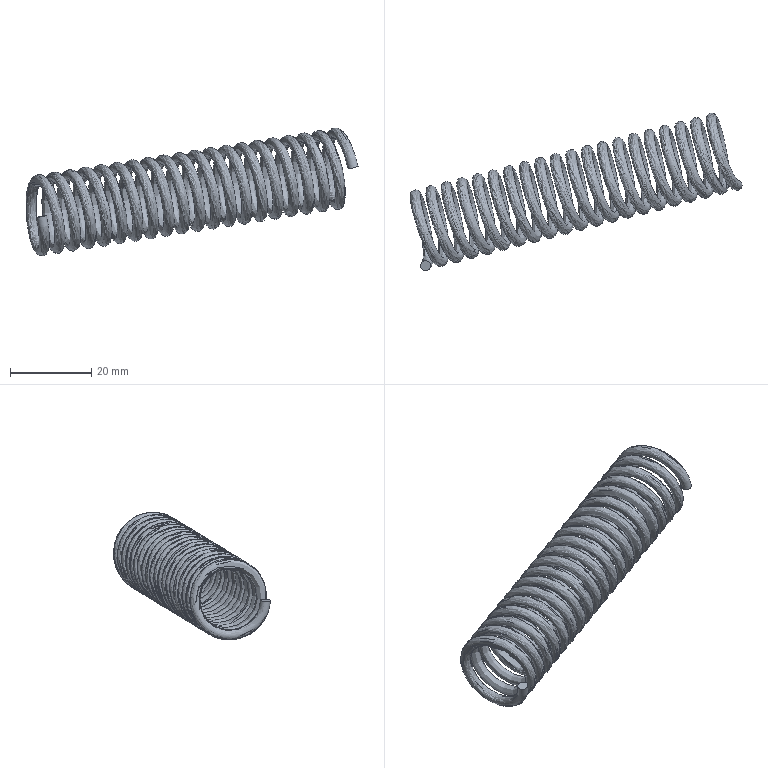Part | STEP file | 车灯-后视镜_id322_x_t | 1 solid | 3 faces | box 81.604 x 38.677 x 31.456 mm | volume 5262 mm3 | plane 2 | spline 1